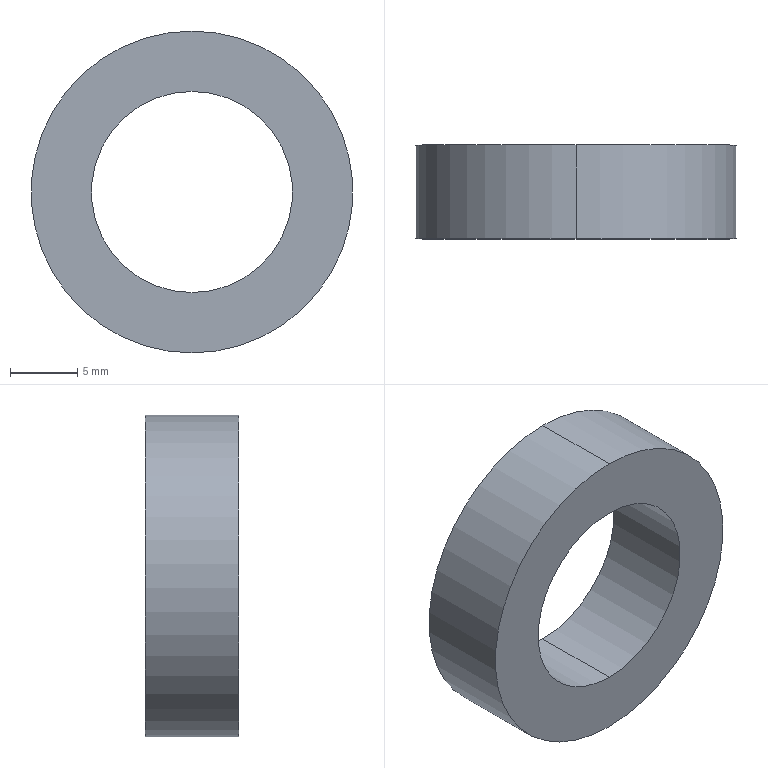Part | SolidWorks | features Extrusion 1 | 1 solid | 6 faces | box 24 x 7 x 24 mm | volume 1930 mm3 | cylinder 4 | plane 2 | commonest cylinder face diameters 15 x2 24 x2
STEP:
#1=CARTESIAN_POINT('',(0.,7.,-7.5));
#2=VERTEX_POINT('',#1);
#3=CARTESIAN_POINT('',(0.,7.,7.5));
#4=VERTEX_POINT('',#3);
#5=CARTESIAN_POINT('',(0.,7.,0.));
#6=DIRECTION('',(0.,1.,0.));
#7=DIRECTION('',(0.,0.,1.));
#8=AXIS2_PLACEMENT_3D('',#5,#6,#7);
#9=CIRCLE('',#8,7.5);
#10=EDGE_CURVE('',#2,#4,#9,.T.);
#11=ORIENTED_EDGE('',*,*,#10,.T.);
#12=CARTESIAN_POINT('',(0.,0.,7.5));
#13=VERTEX_POINT('',#12);
#14=CARTESIAN_POINT('',(0.,7.,7.5));
#15=DIRECTION('',(0.,-1.,0.));
#16=VECTOR('',#15,1000.);
#17=LINE('',#14,#16);
#18=EDGE_CURVE('',#4,#13,#17,.T.);
#19=ORIENTED_EDGE('',*,*,#18,.T.);
#20=CARTESIAN_POINT('',(0.,0.,-7.5));
#21=VERTEX_POINT('',#20);
#22=CARTESIAN_POINT('',(0.,0.,0.));
#23=DIRECTION('',(0.,1.,0.));
#24=DIRECTION('',(0.,0.,1.));
#25=AXIS2_PLACEMENT_3D('',#22,#23,#24);
#26=CIRCLE('',#25,7.5);
#27=EDGE_CURVE('',#21,#13,#26,.T.);
#28=ORIENTED_EDGE('',*,*,#27,.F.);
#29=CARTESIAN_POINT('',(0.,7.,-7.5));
#30=DIRECTION('',(0.,-1.,0.));
#31=VECTOR('',#30,1000.);
#32=LINE('',#29,#31);
#33=EDGE_CURVE('',#2,#21,#32,.T.);
#34=ORIENTED_EDGE('',*,*,#33,.F.);
#35=EDGE_LOOP('',(#11,#19,#28,#34));
#36=FACE_OUTER_BOUND('',#35,.T.);
#37=CARTESIAN_POINT('',(0.,7.,0.));
#38=DIRECTION('',(0.,-1.,0.));
#39=DIRECTION('',(0.,0.,-1.));
#40=AXIS2_PLACEMENT_3D('',#37,#38,#39);
#41=CYLINDRICAL_SURFACE('',#40,7.5);
#42=ADVANCED_FACE('',(#36),#41,.F.);
#43=CARTESIAN_POINT('',(0.,7.,12.));
#44=VERTEX_POINT('',#43);
#45=CARTESIAN_POINT('',(0.,7.,-12.));
#46=VERTEX_POINT('',#45);
#47=CARTESIAN_POINT('',(0.,7.,0.));
#48=DIRECTION('',(0.,1.,0.));
#49=DIRECTION('',(0.,0.,1.));
#50=AXIS2_PLACEMENT_3D('',#47,#48,#49);
#51=CIRCLE('',#50,12.);
#52=EDGE_CURVE('',#44,#46,#51,.T.);
#53=ORIENTED_EDGE('',*,*,#52,.F.);
#54=CARTESIAN_POINT('',(0.,0.,12.));
#55=VERTEX_POINT('',#54);
#56=CARTESIAN_POINT('',(0.,7.,12.));
#57=DIRECTION('',(0.,-1.,0.));
#58=VECTOR('',#57,1000.);
#59=LINE('',#56,#58);
#60=EDGE_CURVE('',#44,#55,#59,.T.);
#61=ORIENTED_EDGE('',*,*,#60,.T.);
#62=CARTESIAN_POINT('',(0.,0.,-12.));
#63=VERTEX_POINT('',#62);
#64=CARTESIAN_POINT('',(0.,0.,0.));
#65=DIRECTION('',(0.,1.,0.));
#66=DIRECTION('',(0.,0.,1.));
#67=AXIS2_PLACEMENT_3D('',#64,#65,#66);
#68=CIRCLE('',#67,12.);
#69=EDGE_CURVE('',#55,#63,#68,.T.);
#70=ORIENTED_EDGE('',*,*,#69,.T.);
#71=CARTESIAN_POINT('',(0.,7.,-12.));
#72=DIRECTION('',(0.,-1.,0.));
#73=VECTOR('',#72,1000.);
#74=LINE('',#71,#73);
#75=EDGE_CURVE('',#46,#63,#74,.T.);
#76=ORIENTED_EDGE('',*,*,#75,.F.);
#77=EDGE_LOOP('',(#53,#61,#70,#76));
#78=FACE_OUTER_BOUND('',#77,.T.);
#79=CARTESIAN_POINT('',(0.,7.,0.));
#80=DIRECTION('',(0.,-1.,0.));
#81=DIRECTION('',(0.,0.,-1.));
#82=AXIS2_PLACEMENT_3D('',#79,#80,#81);
#83=CYLINDRICAL_SURFACE('',#82,12.);
#84=ADVANCED_FACE('',(#78),#83,.T.);
#85=CARTESIAN_POINT('',(0.,7.,0.));
#86=DIRECTION('',(0.,1.,0.));
#87=DIRECTION('',(0.,0.,1.));
#88=AXIS2_PLACEMENT_3D('',#85,#86,#87);
#89=CIRCLE('',#88,12.);
#90=EDGE_CURVE('',#46,#44,#89,.T.);
#91=ORIENTED_EDGE('',*,*,#90,.T.);
#92=ORIENTED_EDGE('',*,*,#52,.T.);
#93=EDGE_LOOP('',(#91,#92));
#94=FACE_OUTER_BOUND('',#93,.T.);
#95=ORIENTED_EDGE('',*,*,#10,.F.);
#96=CARTESIAN_POINT('',(0.,7.,0.));
#97=DIRECTION('',(0.,1.,0.));
#98=DIRECTION('',(0.,0.,1.));
#99=AXIS2_PLACEMENT_3D('',#96,#97,#98);
#100=CIRCLE('',#99,7.5);
#101=EDGE_CURVE('',#4,#2,#100,.T.);
#102=ORIENTED_EDGE('',*,*,#101,.F.);
#103=EDGE_LOOP('',(#95,#102));
#104=FACE_BOUND('',#103,.T.);
#105=CARTESIAN_POINT('',(0.,7.,0.));
#106=DIRECTION('',(0.,1.,0.));
#107=DIRECTION('',(0.,0.,1.));
#108=AXIS2_PLACEMENT_3D('',#105,#106,#107);
#109=PLANE('',#108);
#110=ADVANCED_FACE('',(#94,#104),#109,.T.);
#111=CARTESIAN_POINT('',(0.,0.,0.));
#112=DIRECTION('',(0.,1.,0.));
#113=DIRECTION('',(0.,0.,1.));
#114=AXIS2_PLACEMENT_3D('',#111,#112,#113);
#115=CIRCLE('',#114,12.);
#116=EDGE_CURVE('',#63,#55,#115,.T.);
#117=ORIENTED_EDGE('',*,*,#116,.F.);
#118=ORIENTED_EDGE('',*,*,#69,.F.);
#119=EDGE_LOOP('',(#117,#118));
#120=FACE_OUTER_BOUND('',#119,.T.);
#121=ORIENTED_EDGE('',*,*,#27,.T.);
#122=CARTESIAN_POINT('',(0.,0.,0.));
#123=DIRECTION('',(0.,1.,0.));
#124=DIRECTION('',(0.,0.,1.));
#125=AXIS2_PLACEMENT_3D('',#122,#123,#124);
#126=CIRCLE('',#125,7.5);
#127=EDGE_CURVE('',#13,#21,#126,.T.);
#128=ORIENTED_EDGE('',*,*,#127,.T.);
#129=EDGE_LOOP('',(#121,#128));
#130=FACE_BOUND('',#129,.T.);
#131=CARTESIAN_POINT('',(0.,0.,0.));
#132=DIRECTION('',(0.,1.,0.));
#133=DIRECTION('',(0.,0.,1.));
#134=AXIS2_PLACEMENT_3D('',#131,#132,#133);
#135=PLANE('',#134);
#136=ADVANCED_FACE('',(#120,#130),#135,.F.);
#137=ORIENTED_EDGE('',*,*,#60,.F.);
#138=ORIENTED_EDGE('',*,*,#90,.F.);
#139=ORIENTED_EDGE('',*,*,#75,.T.);
#140=ORIENTED_EDGE('',*,*,#116,.T.);
#141=EDGE_LOOP('',(#137,#138,#139,#140));
#142=FACE_OUTER_BOUND('',#141,.T.);
#143=CARTESIAN_POINT('',(0.,7.,0.));
#144=DIRECTION('',(0.,-1.,0.));
#145=DIRECTION('',(0.,0.,-1.));
#146=AXIS2_PLACEMENT_3D('',#143,#144,#145);
#147=CYLINDRICAL_SURFACE('',#146,12.);
#148=ADVANCED_FACE('',(#142),#147,.T.);
#149=ORIENTED_EDGE('',*,*,#18,.F.);
#150=ORIENTED_EDGE('',*,*,#101,.T.);
#151=ORIENTED_EDGE('',*,*,#33,.T.);
#152=ORIENTED_EDGE('',*,*,#127,.F.);
#153=EDGE_LOOP('',(#149,#150,#151,#152));
#154=FACE_OUTER_BOUND('',#153,.T.);
#155=CARTESIAN_POINT('',(0.,7.,0.));
#156=DIRECTION('',(0.,-1.,0.));
#157=DIRECTION('',(0.,0.,-1.));
#158=AXIS2_PLACEMENT_3D('',#155,#156,#157);
#159=CYLINDRICAL_SURFACE('',#158,7.5);
#160=ADVANCED_FACE('',(#154),#159,.F.);
#161=CLOSED_SHELL('',(#42,#84,#110,#136,#148,#160));
#162=MANIFOLD_SOLID_BREP('',#161);
#163=CARTESIAN_POINT('',(0.,0.,0.));
#164=DIRECTION('',(0.,0.,1.));
#165=DIRECTION('',(1.,0.,0.));
#166=AXIS2_PLACEMENT_3D('',#163,#164,#165);
#167=(LENGTH_UNIT()NAMED_UNIT(*)SI_UNIT(.MILLI.,.METRE.));
#168=UNCERTAINTY_MEASURE_WITH_UNIT(LENGTH_MEASURE(0.00001),#167,'','');
#169=(NAMED_UNIT(*)PLANE_ANGLE_UNIT()SI_UNIT($,.RADIAN.));
#170=(NAMED_UNIT(*)SI_UNIT($,.STERADIAN.)SOLID_ANGLE_UNIT());
#171=(GEOMETRIC_REPRESENTATION_CONTEXT(3)GLOBAL_UNCERTAINTY_ASSIGNED_CONTEXT((#168))GLOBAL_UNIT_ASSIGNED_CONTEXT((#167,#169,#170))REPRESENTATION_CONTEXT('',''));
#172=ADVANCED_BREP_SHAPE_REPRESENTATION('',(#162,#166),#171);